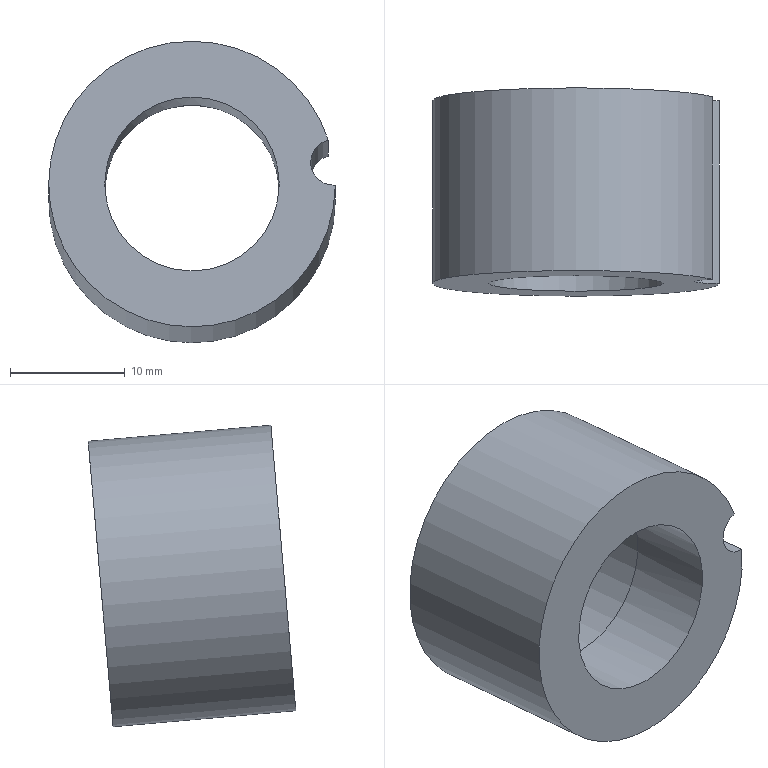Part | NX | features solid 2 | 1 solid | 7 faces | box 25 x 18.118 x 26.299 mm | volume 4570 mm3 | cylinder 4 | plane 3 | commonest cylinder face diameters 4 x1 15.22 x1 16.6 x1 25 x1
STEP:
#1=CARTESIAN_POINT('',(-507.502,-50.065,-20.591));
#2=VERTEX_POINT('',#1);
#3=CARTESIAN_POINT('',(-508.106,-49.722,-16.665));
#4=VERTEX_POINT('',#3);
#5=CARTESIAN_POINT('',(-507.646,-49.892,-18.604));
#6=DIRECTION('',(0.,0.9962,-0.08716));
#7=DIRECTION('',(0.,0.08716,0.9962));
#8=AXIS2_PLACEMENT_3D('',#5,#6,#7);
#9=CIRCLE('',#8,2.);
#10=EDGE_CURVE('',#2,#4,#9,.T.);
#11=ORIENTED_EDGE('',*,*,#10,.T.);
#12=CARTESIAN_POINT('',(-520.002,-50.057,-20.491));
#13=DIRECTION('',(0.,-0.9962,0.08716));
#14=DIRECTION('',(0.,-0.08716,-0.9962));
#15=AXIS2_PLACEMENT_3D('',#12,#13,#14);
#16=CIRCLE('',#15,12.5);
#17=EDGE_CURVE('',#2,#4,#16,.F.);
#18=ORIENTED_EDGE('',*,*,#17,.F.);
#19=EDGE_LOOP('',(#11,#18));
#20=FACE_BOUND('',#19,.T.);
#21=CARTESIAN_POINT('',(-520.002,-49.394,-12.91));
#22=VERTEX_POINT('',#21);
#23=CARTESIAN_POINT('',(-520.002,-50.057,-20.491));
#24=DIRECTION('',(0.,0.9962,-0.08716));
#25=DIRECTION('',(0.,0.08716,0.9962));
#26=AXIS2_PLACEMENT_3D('',#23,#24,#25);
#27=CIRCLE('',#26,7.61);
#28=EDGE_CURVE('',#22,#22,#27,.T.);
#29=ORIENTED_EDGE('',*,*,#28,.T.);
#30=EDGE_LOOP('',(#29));
#31=FACE_BOUND('',#30,.T.);
#32=CARTESIAN_POINT('',(-520.002,-50.057,-20.491));
#33=DIRECTION('',(0.,-0.9962,0.08716));
#34=DIRECTION('',(0.,-0.08716,-0.9962));
#35=AXIS2_PLACEMENT_3D('',#32,#33,#34);
#36=PLANE('',#35);
#37=ADVANCED_FACE('',(#20,#31),#36,.T.);
#38=CARTESIAN_POINT('',(-508.106,-33.783,-18.059));
#39=VERTEX_POINT('',#38);
#40=CARTESIAN_POINT('',(-507.502,-34.126,-21.985));
#41=VERTEX_POINT('',#40);
#42=CARTESIAN_POINT('',(-507.646,-33.953,-19.998));
#43=DIRECTION('',(0.,0.9962,-0.08716));
#44=DIRECTION('',(0.,0.08716,0.9962));
#45=AXIS2_PLACEMENT_3D('',#42,#43,#44);
#46=CIRCLE('',#45,2.);
#47=EDGE_CURVE('',#39,#41,#46,.F.);
#48=ORIENTED_EDGE('',*,*,#47,.T.);
#49=CARTESIAN_POINT('',(-520.002,-34.118,-21.886));
#50=DIRECTION('',(0.,0.9962,-0.08716));
#51=DIRECTION('',(0.,0.08716,0.9962));
#52=AXIS2_PLACEMENT_3D('',#49,#50,#51);
#53=CIRCLE('',#52,12.5);
#54=EDGE_CURVE('',#39,#41,#53,.F.);
#55=ORIENTED_EDGE('',*,*,#54,.F.);
#56=EDGE_LOOP('',(#48,#55));
#57=FACE_BOUND('',#56,.T.);
#58=CARTESIAN_POINT('',(-520.002,-33.394,-13.617));
#59=VERTEX_POINT('',#58);
#60=CARTESIAN_POINT('',(-520.002,-34.118,-21.886));
#61=DIRECTION('',(0.,0.9962,-0.08716));
#62=DIRECTION('',(0.,0.08716,0.9962));
#63=AXIS2_PLACEMENT_3D('',#60,#61,#62);
#64=CIRCLE('',#63,8.3);
#65=EDGE_CURVE('',#59,#59,#64,.F.);
#66=ORIENTED_EDGE('',*,*,#65,.T.);
#67=EDGE_LOOP('',(#66));
#68=FACE_BOUND('',#67,.T.);
#69=CARTESIAN_POINT('',(-520.002,-34.118,-21.886));
#70=DIRECTION('',(0.,0.9962,-0.08716));
#71=DIRECTION('',(0.,0.08716,0.9962));
#72=AXIS2_PLACEMENT_3D('',#69,#70,#71);
#73=PLANE('',#72);
#74=ADVANCED_FACE('',(#57,#68),#73,.T.);
#75=CARTESIAN_POINT('',(-508.106,-41.752,-17.362));
#76=DIRECTION('',(0.,-0.9962,0.08716));
#77=VECTOR('',#76,1000.);
#78=LINE('',#75,#77);
#79=EDGE_CURVE('',#39,#4,#78,.T.);
#80=ORIENTED_EDGE('',*,*,#79,.F.);
#81=ORIENTED_EDGE('',*,*,#54,.T.);
#82=CARTESIAN_POINT('',(-507.502,-42.096,-21.288));
#83=DIRECTION('',(0.,-0.9962,0.08716));
#84=VECTOR('',#83,1000.);
#85=LINE('',#82,#84);
#86=EDGE_CURVE('',#2,#41,#85,.F.);
#87=ORIENTED_EDGE('',*,*,#86,.F.);
#88=ORIENTED_EDGE('',*,*,#17,.T.);
#89=EDGE_LOOP('',(#80,#81,#87,#88));
#90=FACE_BOUND('',#89,.T.);
#91=CARTESIAN_POINT('',(-520.002,-30.133,-22.234));
#92=DIRECTION('',(0.,-0.9962,0.08716));
#93=DIRECTION('',(0.,-0.08716,-0.9962));
#94=AXIS2_PLACEMENT_3D('',#91,#92,#93);
#95=CYLINDRICAL_SURFACE('',#94,12.5);
#96=ADVANCED_FACE('',(#90),#95,.T.);
#97=CARTESIAN_POINT('',(-520.002,-42.75,-28.77));
#98=VERTEX_POINT('',#97);
#99=CARTESIAN_POINT('',(-520.002,-42.087,-21.189));
#100=DIRECTION('',(0.,-0.9962,0.08716));
#101=DIRECTION('',(0.,-0.08716,-0.9962));
#102=AXIS2_PLACEMENT_3D('',#99,#100,#101);
#103=CIRCLE('',#102,7.61);
#104=EDGE_CURVE('',#98,#98,#103,.T.);
#105=ORIENTED_EDGE('',*,*,#104,.T.);
#106=EDGE_LOOP('',(#105));
#107=FACE_BOUND('',#106,.T.);
#108=CARTESIAN_POINT('',(-520.002,-42.811,-29.457));
#109=VERTEX_POINT('',#108);
#110=CARTESIAN_POINT('',(-520.002,-42.087,-21.189));
#111=DIRECTION('',(0.,-0.9962,0.08716));
#112=DIRECTION('',(0.,-0.08716,-0.9962));
#113=AXIS2_PLACEMENT_3D('',#110,#111,#112);
#114=CIRCLE('',#113,8.3);
#115=EDGE_CURVE('',#109,#109,#114,.F.);
#116=ORIENTED_EDGE('',*,*,#115,.T.);
#117=EDGE_LOOP('',(#116));
#118=FACE_BOUND('',#117,.T.);
#119=CARTESIAN_POINT('',(-520.002,-42.087,-21.189));
#120=DIRECTION('',(0.,-0.9962,0.08716));
#121=DIRECTION('',(0.,-0.08716,-0.9962));
#122=AXIS2_PLACEMENT_3D('',#119,#120,#121);
#123=PLANE('',#122);
#124=ADVANCED_FACE('',(#107,#118),#123,.F.);
#125=ORIENTED_EDGE('',*,*,#115,.F.);
#126=EDGE_LOOP('',(#125));
#127=FACE_BOUND('',#126,.T.);
#128=ORIENTED_EDGE('',*,*,#65,.F.);
#129=EDGE_LOOP('',(#128));
#130=FACE_BOUND('',#129,.T.);
#131=CARTESIAN_POINT('',(-520.002,-30.133,-22.234));
#132=DIRECTION('',(0.,-0.9962,0.08716));
#133=DIRECTION('',(0.,-0.08716,-0.9962));
#134=AXIS2_PLACEMENT_3D('',#131,#132,#133);
#135=CYLINDRICAL_SURFACE('',#134,8.3);
#136=ADVANCED_FACE('',(#127,#130),#135,.F.);
#137=ORIENTED_EDGE('',*,*,#28,.F.);
#138=EDGE_LOOP('',(#137));
#139=FACE_BOUND('',#138,.T.);
#140=ORIENTED_EDGE('',*,*,#104,.F.);
#141=EDGE_LOOP('',(#140));
#142=FACE_BOUND('',#141,.T.);
#143=CARTESIAN_POINT('',(-520.002,-42.087,-21.189));
#144=DIRECTION('',(0.,-0.9962,0.08716));
#145=DIRECTION('',(0.,-0.08716,-0.9962));
#146=AXIS2_PLACEMENT_3D('',#143,#144,#145);
#147=CYLINDRICAL_SURFACE('',#146,7.61);
#148=ADVANCED_FACE('',(#139,#142),#147,.F.);
#149=ORIENTED_EDGE('',*,*,#79,.T.);
#150=ORIENTED_EDGE('',*,*,#10,.F.);
#151=ORIENTED_EDGE('',*,*,#86,.T.);
#152=ORIENTED_EDGE('',*,*,#47,.F.);
#153=EDGE_LOOP('',(#149,#150,#151,#152));
#154=FACE_BOUND('',#153,.T.);
#155=CARTESIAN_POINT('',(-507.646,-29.968,-20.347));
#156=DIRECTION('',(0.,-0.9962,0.08716));
#157=DIRECTION('',(0.,-0.08716,-0.9962));
#158=AXIS2_PLACEMENT_3D('',#155,#156,#157);
#159=CYLINDRICAL_SURFACE('',#158,2.);
#160=ADVANCED_FACE('',(#154),#159,.F.);
#161=CLOSED_SHELL('',(#37,#74,#96,#124,#136,#148,#160));
#162=MANIFOLD_SOLID_BREP('',#161);
#163=(LENGTH_UNIT()NAMED_UNIT(*)SI_UNIT(.MILLI.,.METRE.));
#164=UNCERTAINTY_MEASURE_WITH_UNIT(LENGTH_MEASURE(0.00001),#163,'','');
#165=(NAMED_UNIT(*)PLANE_ANGLE_UNIT()SI_UNIT($,.RADIAN.));
#166=(NAMED_UNIT(*)SI_UNIT($,.STERADIAN.)SOLID_ANGLE_UNIT());
#167=(GEOMETRIC_REPRESENTATION_CONTEXT(3)GLOBAL_UNCERTAINTY_ASSIGNED_CONTEXT((#164))GLOBAL_UNIT_ASSIGNED_CONTEXT((#163,#165,#166))REPRESENTATION_CONTEXT('',''));
#168=ADVANCED_BREP_SHAPE_REPRESENTATION('',(#162),#167);